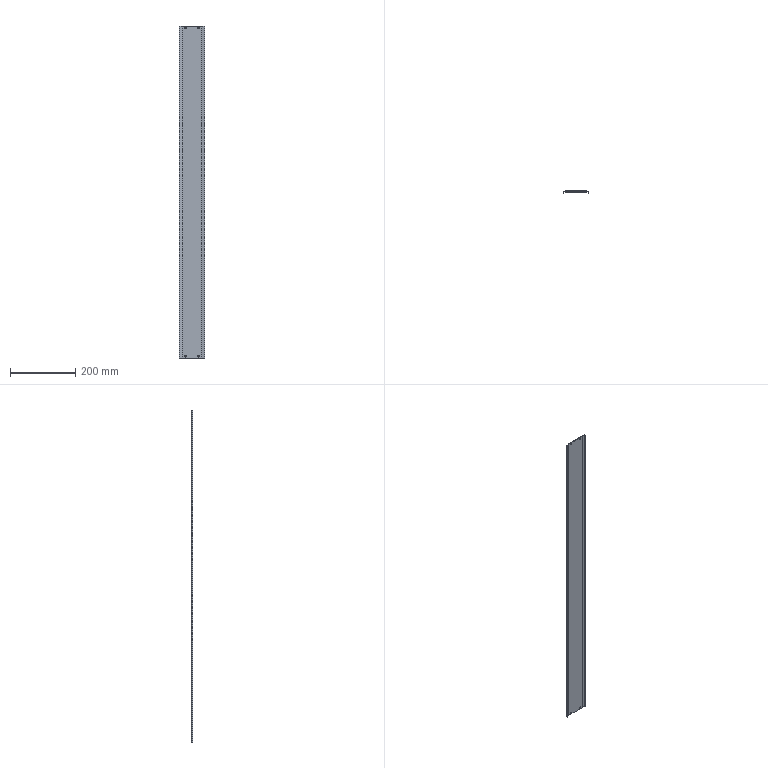Part | SolidWorks | features Cut 1, Extrusion 1, MirrorPattern 1 | 1 solid | 22 faces | box 79 x 6 x 1020 mm | volume 209920 mm3 | plane 14 | cylinder 8 | commonest cylinder face diameters 4.5 x8
STEP:
#1=CARTESIAN_POINT('',(20.,3.5,507.25));
#2=VERTEX_POINT('',#1);
#3=CARTESIAN_POINT('',(20.,3.5,502.75));
#4=VERTEX_POINT('',#3);
#5=CARTESIAN_POINT('',(20.,3.5,505.));
#6=DIRECTION('',(0.,-1.,0.));
#7=DIRECTION('',(0.,0.,1.));
#8=AXIS2_PLACEMENT_3D('',#5,#6,#7);
#9=CIRCLE('',#8,2.25);
#10=EDGE_CURVE('',#2,#4,#9,.T.);
#11=ORIENTED_EDGE('',*,*,#10,.T.);
#12=CARTESIAN_POINT('',(20.,6.,502.75));
#13=VERTEX_POINT('',#12);
#14=CARTESIAN_POINT('',(20.,-14.,502.75));
#15=DIRECTION('',(0.,1.,0.));
#16=VECTOR('',#15,1000.);
#17=LINE('',#14,#16);
#18=EDGE_CURVE('',#4,#13,#17,.T.);
#19=ORIENTED_EDGE('',*,*,#18,.T.);
#20=CARTESIAN_POINT('',(20.,6.,507.25));
#21=VERTEX_POINT('',#20);
#22=CARTESIAN_POINT('',(20.,6.,505.));
#23=DIRECTION('',(0.,-1.,0.));
#24=DIRECTION('',(0.,0.,-1.));
#25=AXIS2_PLACEMENT_3D('',#22,#23,#24);
#26=CIRCLE('',#25,2.25);
#27=EDGE_CURVE('',#21,#13,#26,.T.);
#28=ORIENTED_EDGE('',*,*,#27,.F.);
#29=CARTESIAN_POINT('',(20.,-14.,507.25));
#30=DIRECTION('',(0.,1.,0.));
#31=VECTOR('',#30,1000.);
#32=LINE('',#29,#31);
#33=EDGE_CURVE('',#2,#21,#32,.T.);
#34=ORIENTED_EDGE('',*,*,#33,.F.);
#35=EDGE_LOOP('',(#11,#19,#28,#34));
#36=FACE_OUTER_BOUND('',#35,.T.);
#37=CARTESIAN_POINT('',(20.,-14.,505.));
#38=DIRECTION('',(0.,1.,0.));
#39=DIRECTION('',(0.,0.,1.));
#40=AXIS2_PLACEMENT_3D('',#37,#38,#39);
#41=CYLINDRICAL_SURFACE('',#40,2.25);
#42=ADVANCED_FACE('',(#36),#41,.F.);
#43=CARTESIAN_POINT('',(-20.,3.5,507.25));
#44=VERTEX_POINT('',#43);
#45=CARTESIAN_POINT('',(-20.,3.5,502.75));
#46=VERTEX_POINT('',#45);
#47=CARTESIAN_POINT('',(-20.,3.5,505.));
#48=DIRECTION('',(0.,-1.,0.));
#49=DIRECTION('',(0.,0.,1.));
#50=AXIS2_PLACEMENT_3D('',#47,#48,#49);
#51=CIRCLE('',#50,2.25);
#52=EDGE_CURVE('',#44,#46,#51,.T.);
#53=ORIENTED_EDGE('',*,*,#52,.T.);
#54=CARTESIAN_POINT('',(-20.,6.,502.75));
#55=VERTEX_POINT('',#54);
#56=CARTESIAN_POINT('',(-20.,-14.,502.75));
#57=DIRECTION('',(0.,1.,0.));
#58=VECTOR('',#57,1000.);
#59=LINE('',#56,#58);
#60=EDGE_CURVE('',#46,#55,#59,.T.);
#61=ORIENTED_EDGE('',*,*,#60,.T.);
#62=CARTESIAN_POINT('',(-20.,6.,507.25));
#63=VERTEX_POINT('',#62);
#64=CARTESIAN_POINT('',(-20.,6.,505.));
#65=DIRECTION('',(0.,-1.,0.));
#66=DIRECTION('',(0.,0.,-1.));
#67=AXIS2_PLACEMENT_3D('',#64,#65,#66);
#68=CIRCLE('',#67,2.25);
#69=EDGE_CURVE('',#63,#55,#68,.T.);
#70=ORIENTED_EDGE('',*,*,#69,.F.);
#71=CARTESIAN_POINT('',(-20.,-14.,507.25));
#72=DIRECTION('',(0.,1.,0.));
#73=VECTOR('',#72,1000.);
#74=LINE('',#71,#73);
#75=EDGE_CURVE('',#44,#63,#74,.T.);
#76=ORIENTED_EDGE('',*,*,#75,.F.);
#77=EDGE_LOOP('',(#53,#61,#70,#76));
#78=FACE_OUTER_BOUND('',#77,.T.);
#79=CARTESIAN_POINT('',(-20.,-14.,505.));
#80=DIRECTION('',(0.,1.,0.));
#81=DIRECTION('',(0.,0.,1.));
#82=AXIS2_PLACEMENT_3D('',#79,#80,#81);
#83=CYLINDRICAL_SURFACE('',#82,2.25);
#84=ADVANCED_FACE('',(#78),#83,.F.);
#85=CARTESIAN_POINT('',(20.,3.5,-507.25));
#86=VERTEX_POINT('',#85);
#87=CARTESIAN_POINT('',(20.,3.5,-502.75));
#88=VERTEX_POINT('',#87);
#89=CARTESIAN_POINT('',(20.,3.5,-505.));
#90=DIRECTION('',(0.,1.,0.));
#91=DIRECTION('',(0.,0.,1.));
#92=AXIS2_PLACEMENT_3D('',#89,#90,#91);
#93=CIRCLE('',#92,2.25);
#94=EDGE_CURVE('',#86,#88,#93,.T.);
#95=ORIENTED_EDGE('',*,*,#94,.F.);
#96=CARTESIAN_POINT('',(20.,6.,-507.25));
#97=VERTEX_POINT('',#96);
#98=CARTESIAN_POINT('',(20.,-14.,-507.25));
#99=DIRECTION('',(0.,1.,0.));
#100=VECTOR('',#99,1000.);
#101=LINE('',#98,#100);
#102=EDGE_CURVE('',#86,#97,#101,.T.);
#103=ORIENTED_EDGE('',*,*,#102,.T.);
#104=CARTESIAN_POINT('',(20.,6.,-502.75));
#105=VERTEX_POINT('',#104);
#106=CARTESIAN_POINT('',(20.,6.,-505.));
#107=DIRECTION('',(0.,1.,0.));
#108=DIRECTION('',(0.,0.,1.));
#109=AXIS2_PLACEMENT_3D('',#106,#107,#108);
#110=CIRCLE('',#109,2.25);
#111=EDGE_CURVE('',#97,#105,#110,.T.);
#112=ORIENTED_EDGE('',*,*,#111,.T.);
#113=CARTESIAN_POINT('',(20.,-14.,-502.75));
#114=DIRECTION('',(0.,1.,0.));
#115=VECTOR('',#114,1000.);
#116=LINE('',#113,#115);
#117=EDGE_CURVE('',#88,#105,#116,.T.);
#118=ORIENTED_EDGE('',*,*,#117,.F.);
#119=EDGE_LOOP('',(#95,#103,#112,#118));
#120=FACE_OUTER_BOUND('',#119,.T.);
#121=CARTESIAN_POINT('',(20.,-14.,-505.));
#122=DIRECTION('',(0.,1.,0.));
#123=DIRECTION('',(0.,0.,1.));
#124=AXIS2_PLACEMENT_3D('',#121,#122,#123);
#125=CYLINDRICAL_SURFACE('',#124,2.25);
#126=ADVANCED_FACE('',(#120),#125,.F.);
#127=CARTESIAN_POINT('',(-20.,3.5,-507.25));
#128=VERTEX_POINT('',#127);
#129=CARTESIAN_POINT('',(-20.,3.5,-502.75));
#130=VERTEX_POINT('',#129);
#131=CARTESIAN_POINT('',(-20.,3.5,-505.));
#132=DIRECTION('',(0.,1.,0.));
#133=DIRECTION('',(0.,0.,1.));
#134=AXIS2_PLACEMENT_3D('',#131,#132,#133);
#135=CIRCLE('',#134,2.25);
#136=EDGE_CURVE('',#128,#130,#135,.T.);
#137=ORIENTED_EDGE('',*,*,#136,.F.);
#138=CARTESIAN_POINT('',(-20.,6.,-507.25));
#139=VERTEX_POINT('',#138);
#140=CARTESIAN_POINT('',(-20.,-14.,-507.25));
#141=DIRECTION('',(0.,1.,0.));
#142=VECTOR('',#141,1000.);
#143=LINE('',#140,#142);
#144=EDGE_CURVE('',#128,#139,#143,.T.);
#145=ORIENTED_EDGE('',*,*,#144,.T.);
#146=CARTESIAN_POINT('',(-20.,6.,-502.75));
#147=VERTEX_POINT('',#146);
#148=CARTESIAN_POINT('',(-20.,6.,-505.));
#149=DIRECTION('',(0.,1.,0.));
#150=DIRECTION('',(0.,0.,1.));
#151=AXIS2_PLACEMENT_3D('',#148,#149,#150);
#152=CIRCLE('',#151,2.25);
#153=EDGE_CURVE('',#139,#147,#152,.T.);
#154=ORIENTED_EDGE('',*,*,#153,.T.);
#155=CARTESIAN_POINT('',(-20.,-14.,-502.75));
#156=DIRECTION('',(0.,1.,0.));
#157=VECTOR('',#156,1000.);
#158=LINE('',#155,#157);
#159=EDGE_CURVE('',#130,#147,#158,.T.);
#160=ORIENTED_EDGE('',*,*,#159,.F.);
#161=EDGE_LOOP('',(#137,#145,#154,#160));
#162=FACE_OUTER_BOUND('',#161,.T.);
#163=CARTESIAN_POINT('',(-20.,-14.,-505.));
#164=DIRECTION('',(0.,1.,0.));
#165=DIRECTION('',(0.,0.,1.));
#166=AXIS2_PLACEMENT_3D('',#163,#164,#165);
#167=CYLINDRICAL_SURFACE('',#166,2.25);
#168=ADVANCED_FACE('',(#162),#167,.F.);
#169=CARTESIAN_POINT('',(-37.5,0.,-510.));
#170=VERTEX_POINT('',#169);
#171=CARTESIAN_POINT('',(-37.5,2.122,-510.));
#172=VERTEX_POINT('',#171);
#173=CARTESIAN_POINT('',(-37.5,0.,-510.));
#174=DIRECTION('',(0.,1.,0.));
#175=VECTOR('',#174,1000.);
#176=LINE('',#173,#175);
#177=EDGE_CURVE('',#170,#172,#176,.T.);
#178=ORIENTED_EDGE('',*,*,#177,.T.);
#179=CARTESIAN_POINT('',(-37.5,2.122,510.));
#180=VERTEX_POINT('',#179);
#181=CARTESIAN_POINT('',(-37.5,2.122,510.));
#182=DIRECTION('',(0.,0.,-1.));
#183=VECTOR('',#182,1000.);
#184=LINE('',#181,#183);
#185=EDGE_CURVE('',#180,#172,#184,.T.);
#186=ORIENTED_EDGE('',*,*,#185,.F.);
#187=CARTESIAN_POINT('',(-37.5,0.,510.));
#188=VERTEX_POINT('',#187);
#189=CARTESIAN_POINT('',(-37.5,0.,510.));
#190=DIRECTION('',(0.,1.,0.));
#191=VECTOR('',#190,1000.);
#192=LINE('',#189,#191);
#193=EDGE_CURVE('',#188,#180,#192,.T.);
#194=ORIENTED_EDGE('',*,*,#193,.F.);
#195=CARTESIAN_POINT('',(-37.5,0.,510.));
#196=DIRECTION('',(0.,0.,-1.));
#197=VECTOR('',#196,1000.);
#198=LINE('',#195,#197);
#199=EDGE_CURVE('',#188,#170,#198,.T.);
#200=ORIENTED_EDGE('',*,*,#199,.T.);
#201=EDGE_LOOP('',(#178,#186,#194,#200));
#202=FACE_OUTER_BOUND('',#201,.T.);
#203=CARTESIAN_POINT('',(-37.5,0.,510.));
#204=DIRECTION('',(-1.,0.,0.));
#205=DIRECTION('',(0.,0.,1.));
#206=AXIS2_PLACEMENT_3D('',#203,#204,#205);
#207=PLANE('',#206);
#208=ADVANCED_FACE('',(#202),#207,.F.);
#209=CARTESIAN_POINT('',(-29.8,3.5,-510.));
#210=VERTEX_POINT('',#209);
#211=CARTESIAN_POINT('',(-37.5,2.122,-510.));
#212=DIRECTION('',(0.9844,0.1761,0.));
#213=VECTOR('',#212,1000.);
#214=LINE('',#211,#213);
#215=EDGE_CURVE('',#172,#210,#214,.T.);
#216=ORIENTED_EDGE('',*,*,#215,.T.);
#217=CARTESIAN_POINT('',(-29.8,3.5,510.));
#218=VERTEX_POINT('',#217);
#219=CARTESIAN_POINT('',(-29.8,3.5,510.));
#220=DIRECTION('',(0.,0.,-1.));
#221=VECTOR('',#220,1000.);
#222=LINE('',#219,#221);
#223=EDGE_CURVE('',#218,#210,#222,.T.);
#224=ORIENTED_EDGE('',*,*,#223,.F.);
#225=CARTESIAN_POINT('',(-37.5,2.122,510.));
#226=DIRECTION('',(0.9844,0.1761,0.));
#227=VECTOR('',#226,1000.);
#228=LINE('',#225,#227);
#229=EDGE_CURVE('',#180,#218,#228,.T.);
#230=ORIENTED_EDGE('',*,*,#229,.F.);
#231=ORIENTED_EDGE('',*,*,#185,.T.);
#232=EDGE_LOOP('',(#216,#224,#230,#231));
#233=FACE_OUTER_BOUND('',#232,.T.);
#234=CARTESIAN_POINT('',(-37.5,2.122,510.));
#235=DIRECTION('',(-0.1761,0.9844,0.));
#236=DIRECTION('',(-0.9844,-0.1761,0.));
#237=AXIS2_PLACEMENT_3D('',#234,#235,#236);
#238=PLANE('',#237);
#239=ADVANCED_FACE('',(#233),#238,.F.);
#240=ORIENTED_EDGE('',*,*,#10,.F.);
#241=CARTESIAN_POINT('',(20.,3.5,505.));
#242=DIRECTION('',(0.,-1.,0.));
#243=DIRECTION('',(0.,0.,1.));
#244=AXIS2_PLACEMENT_3D('',#241,#242,#243);
#245=CIRCLE('',#244,2.25);
#246=EDGE_CURVE('',#4,#2,#245,.T.);
#247=ORIENTED_EDGE('',*,*,#246,.F.);
#248=EDGE_LOOP('',(#240,#247));
#249=FACE_BOUND('',#248,.T.);
#250=ORIENTED_EDGE('',*,*,#52,.F.);
#251=CARTESIAN_POINT('',(-20.,3.5,505.));
#252=DIRECTION('',(0.,-1.,0.));
#253=DIRECTION('',(0.,0.,1.));
#254=AXIS2_PLACEMENT_3D('',#251,#252,#253);
#255=CIRCLE('',#254,2.25);
#256=EDGE_CURVE('',#46,#44,#255,.T.);
#257=ORIENTED_EDGE('',*,*,#256,.F.);
#258=EDGE_LOOP('',(#250,#257));
#259=FACE_BOUND('',#258,.T.);
#260=CARTESIAN_POINT('',(20.,3.5,-505.));
#261=DIRECTION('',(0.,1.,0.));
#262=DIRECTION('',(0.,0.,1.));
#263=AXIS2_PLACEMENT_3D('',#260,#261,#262);
#264=CIRCLE('',#263,2.25);
#265=EDGE_CURVE('',#88,#86,#264,.T.);
#266=ORIENTED_EDGE('',*,*,#265,.T.);
#267=ORIENTED_EDGE('',*,*,#94,.T.);
#268=EDGE_LOOP('',(#266,#267));
#269=FACE_BOUND('',#268,.T.);
#270=CARTESIAN_POINT('',(-20.,3.5,-505.));
#271=DIRECTION('',(0.,1.,0.));
#272=DIRECTION('',(0.,0.,1.));
#273=AXIS2_PLACEMENT_3D('',#270,#271,#272);
#274=CIRCLE('',#273,2.25);
#275=EDGE_CURVE('',#130,#128,#274,.T.);
#276=ORIENTED_EDGE('',*,*,#275,.T.);
#277=ORIENTED_EDGE('',*,*,#136,.T.);
#278=EDGE_LOOP('',(#276,#277));
#279=FACE_BOUND('',#278,.T.);
#280=CARTESIAN_POINT('',(29.8,3.5,-510.));
#281=VERTEX_POINT('',#280);
#282=CARTESIAN_POINT('',(-29.8,3.5,-510.));
#283=DIRECTION('',(1.,0.,0.));
#284=VECTOR('',#283,1000.);
#285=LINE('',#282,#284);
#286=EDGE_CURVE('',#210,#281,#285,.T.);
#287=ORIENTED_EDGE('',*,*,#286,.T.);
#288=CARTESIAN_POINT('',(29.8,3.5,510.));
#289=VERTEX_POINT('',#288);
#290=CARTESIAN_POINT('',(29.8,3.5,510.));
#291=DIRECTION('',(0.,0.,-1.));
#292=VECTOR('',#291,1000.);
#293=LINE('',#290,#292);
#294=EDGE_CURVE('',#289,#281,#293,.T.);
#295=ORIENTED_EDGE('',*,*,#294,.F.);
#296=CARTESIAN_POINT('',(-29.8,3.5,510.));
#297=DIRECTION('',(1.,0.,0.));
#298=VECTOR('',#297,1000.);
#299=LINE('',#296,#298);
#300=EDGE_CURVE('',#218,#289,#299,.T.);
#301=ORIENTED_EDGE('',*,*,#300,.F.);
#302=ORIENTED_EDGE('',*,*,#223,.T.);
#303=EDGE_LOOP('',(#287,#295,#301,#302));
#304=FACE_OUTER_BOUND('',#303,.T.);
#305=CARTESIAN_POINT('',(-29.8,3.5,510.));
#306=DIRECTION('',(0.,1.,0.));
#307=DIRECTION('',(0.,0.,1.));
#308=AXIS2_PLACEMENT_3D('',#305,#306,#307);
#309=PLANE('',#308);
#310=ADVANCED_FACE('',(#249,#259,#269,#279,#304),#309,.F.);
#311=CARTESIAN_POINT('',(37.5,2.122,-510.));
#312=VERTEX_POINT('',#311);
#313=CARTESIAN_POINT('',(37.5,2.122,-510.));
#314=DIRECTION('',(0.9844,-0.1761,0.));
#315=VECTOR('',#314,1000.);
#316=LINE('',#313,#315);
#317=EDGE_CURVE('',#281,#312,#316,.T.);
#318=ORIENTED_EDGE('',*,*,#317,.T.);
#319=CARTESIAN_POINT('',(37.5,2.122,510.));
#320=VERTEX_POINT('',#319);
#321=CARTESIAN_POINT('',(37.5,2.122,510.));
#322=DIRECTION('',(0.,0.,-1.));
#323=VECTOR('',#322,1000.);
#324=LINE('',#321,#323);
#325=EDGE_CURVE('',#320,#312,#324,.T.);
#326=ORIENTED_EDGE('',*,*,#325,.F.);
#327=CARTESIAN_POINT('',(37.5,2.122,510.));
#328=DIRECTION('',(0.9844,-0.1761,0.));
#329=VECTOR('',#328,1000.);
#330=LINE('',#327,#329);
#331=EDGE_CURVE('',#289,#320,#330,.T.);
#332=ORIENTED_EDGE('',*,*,#331,.F.);
#333=ORIENTED_EDGE('',*,*,#294,.T.);
#334=EDGE_LOOP('',(#318,#326,#332,#333));
#335=FACE_OUTER_BOUND('',#334,.T.);
#336=CARTESIAN_POINT('',(37.5,2.122,510.));
#337=DIRECTION('',(0.1761,0.9844,0.));
#338=DIRECTION('',(-0.9844,0.1761,0.));
#339=AXIS2_PLACEMENT_3D('',#336,#337,#338);
#340=PLANE('',#339);
#341=ADVANCED_FACE('',(#335),#340,.F.);
#342=CARTESIAN_POINT('',(37.5,0.,-510.));
#343=VERTEX_POINT('',#342);
#344=CARTESIAN_POINT('',(37.5,0.,-510.));
#345=DIRECTION('',(0.,-1.,0.));
#346=VECTOR('',#345,1000.);
#347=LINE('',#344,#346);
#348=EDGE_CURVE('',#312,#343,#347,.T.);
#349=ORIENTED_EDGE('',*,*,#348,.T.);
#350=CARTESIAN_POINT('',(37.5,0.,510.));
#351=VERTEX_POINT('',#350);
#352=CARTESIAN_POINT('',(37.5,0.,510.));
#353=DIRECTION('',(0.,0.,-1.));
#354=VECTOR('',#353,1000.);
#355=LINE('',#352,#354);
#356=EDGE_CURVE('',#351,#343,#355,.T.);
#357=ORIENTED_EDGE('',*,*,#356,.F.);
#358=CARTESIAN_POINT('',(37.5,0.,510.));
#359=DIRECTION('',(0.,-1.,0.));
#360=VECTOR('',#359,1000.);
#361=LINE('',#358,#360);
#362=EDGE_CURVE('',#320,#351,#361,.T.);
#363=ORIENTED_EDGE('',*,*,#362,.F.);
#364=ORIENTED_EDGE('',*,*,#325,.T.);
#365=EDGE_LOOP('',(#349,#357,#363,#364));
#366=FACE_OUTER_BOUND('',#365,.T.);
#367=CARTESIAN_POINT('',(37.5,0.,510.));
#368=DIRECTION('',(1.,0.,0.));
#369=DIRECTION('',(0.,0.,-1.));
#370=AXIS2_PLACEMENT_3D('',#367,#368,#369);
#371=PLANE('',#370);
#372=ADVANCED_FACE('',(#366),#371,.F.);
#373=CARTESIAN_POINT('',(39.5,0.,-510.));
#374=VERTEX_POINT('',#373);
#375=CARTESIAN_POINT('',(37.5,0.,-510.));
#376=DIRECTION('',(1.,0.,0.));
#377=VECTOR('',#376,1000.);
#378=LINE('',#375,#377);
#379=EDGE_CURVE('',#343,#374,#378,.T.);
#380=ORIENTED_EDGE('',*,*,#379,.T.);
#381=CARTESIAN_POINT('',(39.5,0.,510.));
#382=VERTEX_POINT('',#381);
#383=CARTESIAN_POINT('',(39.5,0.,510.));
#384=DIRECTION('',(0.,0.,-1.));
#385=VECTOR('',#384,1000.);
#386=LINE('',#383,#385);
#387=EDGE_CURVE('',#382,#374,#386,.T.);
#388=ORIENTED_EDGE('',*,*,#387,.F.);
#389=CARTESIAN_POINT('',(37.5,0.,510.));
#390=DIRECTION('',(1.,0.,0.));
#391=VECTOR('',#390,1000.);
#392=LINE('',#389,#391);
#393=EDGE_CURVE('',#351,#382,#392,.T.);
#394=ORIENTED_EDGE('',*,*,#393,.F.);
#395=ORIENTED_EDGE('',*,*,#356,.T.);
#396=EDGE_LOOP('',(#380,#388,#394,#395));
#397=FACE_OUTER_BOUND('',#396,.T.);
#398=CARTESIAN_POINT('',(37.5,0.,510.));
#399=DIRECTION('',(0.,1.,0.));
#400=DIRECTION('',(-1.,0.,0.));
#401=AXIS2_PLACEMENT_3D('',#398,#399,#400);
#402=PLANE('',#401);
#403=ADVANCED_FACE('',(#397),#402,.F.);
#404=CARTESIAN_POINT('',(39.5,4.3,-510.));
#405=VERTEX_POINT('',#404);
#406=CARTESIAN_POINT('',(39.5,0.,-510.));
#407=DIRECTION('',(0.,1.,0.));
#408=VECTOR('',#407,1000.);
#409=LINE('',#406,#408);
#410=EDGE_CURVE('',#374,#405,#409,.T.);
#411=ORIENTED_EDGE('',*,*,#410,.T.);
#412=CARTESIAN_POINT('',(39.5,4.3,510.));
#413=VERTEX_POINT('',#412);
#414=CARTESIAN_POINT('',(39.5,4.3,510.));
#415=DIRECTION('',(0.,0.,-1.));
#416=VECTOR('',#415,1000.);
#417=LINE('',#414,#416);
#418=EDGE_CURVE('',#413,#405,#417,.T.);
#419=ORIENTED_EDGE('',*,*,#418,.F.);
#420=CARTESIAN_POINT('',(39.5,0.,510.));
#421=DIRECTION('',(0.,1.,0.));
#422=VECTOR('',#421,1000.);
#423=LINE('',#420,#422);
#424=EDGE_CURVE('',#382,#413,#423,.T.);
#425=ORIENTED_EDGE('',*,*,#424,.F.);
#426=ORIENTED_EDGE('',*,*,#387,.T.);
#427=EDGE_LOOP('',(#411,#419,#425,#426));
#428=FACE_OUTER_BOUND('',#427,.T.);
#429=CARTESIAN_POINT('',(39.5,0.,510.));
#430=DIRECTION('',(-1.,0.,0.));
#431=DIRECTION('',(0.,0.,1.));
#432=AXIS2_PLACEMENT_3D('',#429,#430,#431);
#433=PLANE('',#432);
#434=ADVANCED_FACE('',(#428),#433,.F.);
#435=CARTESIAN_POINT('',(30.,6.,-510.));
#436=VERTEX_POINT('',#435);
#437=CARTESIAN_POINT('',(39.5,4.3,-510.));
#438=DIRECTION('',(-0.9844,0.1761,0.));
#439=VECTOR('',#438,1000.);
#440=LINE('',#437,#439);
#441=EDGE_CURVE('',#405,#436,#440,.T.);
#442=ORIENTED_EDGE('',*,*,#441,.T.);
#443=CARTESIAN_POINT('',(30.,6.,510.));
#444=VERTEX_POINT('',#443);
#445=CARTESIAN_POINT('',(30.,6.,510.));
#446=DIRECTION('',(0.,0.,-1.));
#447=VECTOR('',#446,1000.);
#448=LINE('',#445,#447);
#449=EDGE_CURVE('',#444,#436,#448,.T.);
#450=ORIENTED_EDGE('',*,*,#449,.F.);
#451=CARTESIAN_POINT('',(39.5,4.3,510.));
#452=DIRECTION('',(-0.9844,0.1761,0.));
#453=VECTOR('',#452,1000.);
#454=LINE('',#451,#453);
#455=EDGE_CURVE('',#413,#444,#454,.T.);
#456=ORIENTED_EDGE('',*,*,#455,.F.);
#457=ORIENTED_EDGE('',*,*,#418,.T.);
#458=EDGE_LOOP('',(#442,#450,#456,#457));
#459=FACE_OUTER_BOUND('',#458,.T.);
#460=CARTESIAN_POINT('',(39.5,4.3,510.));
#461=DIRECTION('',(-0.1761,-0.9844,0.));
#462=DIRECTION('',(0.9844,-0.1761,0.));
#463=AXIS2_PLACEMENT_3D('',#460,#461,#462);
#464=PLANE('',#463);
#465=ADVANCED_FACE('',(#459),#464,.F.);
#466=ORIENTED_EDGE('',*,*,#27,.T.);
#467=CARTESIAN_POINT('',(20.,6.,505.));
#468=DIRECTION('',(0.,-1.,0.));
#469=DIRECTION('',(0.,0.,-1.));
#470=AXIS2_PLACEMENT_3D('',#467,#468,#469);
#471=CIRCLE('',#470,2.25);
#472=EDGE_CURVE('',#13,#21,#471,.T.);
#473=ORIENTED_EDGE('',*,*,#472,.T.);
#474=EDGE_LOOP('',(#466,#473));
#475=FACE_BOUND('',#474,.T.);
#476=ORIENTED_EDGE('',*,*,#69,.T.);
#477=CARTESIAN_POINT('',(-20.,6.,505.));
#478=DIRECTION('',(0.,-1.,0.));
#479=DIRECTION('',(0.,0.,-1.));
#480=AXIS2_PLACEMENT_3D('',#477,#478,#479);
#481=CIRCLE('',#480,2.25);
#482=EDGE_CURVE('',#55,#63,#481,.T.);
#483=ORIENTED_EDGE('',*,*,#482,.T.);
#484=EDGE_LOOP('',(#476,#483));
#485=FACE_BOUND('',#484,.T.);
#486=CARTESIAN_POINT('',(20.,6.,-505.));
#487=DIRECTION('',(0.,1.,0.));
#488=DIRECTION('',(0.,0.,1.));
#489=AXIS2_PLACEMENT_3D('',#486,#487,#488);
#490=CIRCLE('',#489,2.25);
#491=EDGE_CURVE('',#105,#97,#490,.T.);
#492=ORIENTED_EDGE('',*,*,#491,.F.);
#493=ORIENTED_EDGE('',*,*,#111,.F.);
#494=EDGE_LOOP('',(#492,#493));
#495=FACE_BOUND('',#494,.T.);
#496=CARTESIAN_POINT('',(-20.,6.,-505.));
#497=DIRECTION('',(0.,1.,0.));
#498=DIRECTION('',(0.,0.,1.));
#499=AXIS2_PLACEMENT_3D('',#496,#497,#498);
#500=CIRCLE('',#499,2.25);
#501=EDGE_CURVE('',#147,#139,#500,.T.);
#502=ORIENTED_EDGE('',*,*,#501,.F.);
#503=ORIENTED_EDGE('',*,*,#153,.F.);
#504=EDGE_LOOP('',(#502,#503));
#505=FACE_BOUND('',#504,.T.);
#506=CARTESIAN_POINT('',(-30.,6.,-510.));
#507=VERTEX_POINT('',#506);
#508=CARTESIAN_POINT('',(-30.,6.,-510.));
#509=DIRECTION('',(-1.,0.,0.));
#510=VECTOR('',#509,1000.);
#511=LINE('',#508,#510);
#512=EDGE_CURVE('',#436,#507,#511,.T.);
#513=ORIENTED_EDGE('',*,*,#512,.T.);
#514=CARTESIAN_POINT('',(-30.,6.,510.));
#515=VERTEX_POINT('',#514);
#516=CARTESIAN_POINT('',(-30.,6.,510.));
#517=DIRECTION('',(0.,0.,-1.));
#518=VECTOR('',#517,1000.);
#519=LINE('',#516,#518);
#520=EDGE_CURVE('',#515,#507,#519,.T.);
#521=ORIENTED_EDGE('',*,*,#520,.F.);
#522=CARTESIAN_POINT('',(-30.,6.,510.));
#523=DIRECTION('',(-1.,0.,0.));
#524=VECTOR('',#523,1000.);
#525=LINE('',#522,#524);
#526=EDGE_CURVE('',#444,#515,#525,.T.);
#527=ORIENTED_EDGE('',*,*,#526,.F.);
#528=ORIENTED_EDGE('',*,*,#449,.T.);
#529=EDGE_LOOP('',(#513,#521,#527,#528));
#530=FACE_OUTER_BOUND('',#529,.T.);
#531=CARTESIAN_POINT('',(-30.,6.,510.));
#532=DIRECTION('',(0.,-1.,0.));
#533=DIRECTION('',(0.,0.,-1.));
#534=AXIS2_PLACEMENT_3D('',#531,#532,#533);
#535=PLANE('',#534);
#536=ADVANCED_FACE('',(#475,#485,#495,#505,#530),#535,.F.);
#537=CARTESIAN_POINT('',(-39.5,4.3,-510.));
#538=VERTEX_POINT('',#537);
#539=CARTESIAN_POINT('',(-39.5,4.3,-510.));
#540=DIRECTION('',(-0.9844,-0.1761,0.));
#541=VECTOR('',#540,1000.);
#542=LINE('',#539,#541);
#543=EDGE_CURVE('',#507,#538,#542,.T.);
#544=ORIENTED_EDGE('',*,*,#543,.T.);
#545=CARTESIAN_POINT('',(-39.5,4.3,510.));
#546=VERTEX_POINT('',#545);
#547=CARTESIAN_POINT('',(-39.5,4.3,510.));
#548=DIRECTION('',(0.,0.,-1.));
#549=VECTOR('',#548,1000.);
#550=LINE('',#547,#549);
#551=EDGE_CURVE('',#546,#538,#550,.T.);
#552=ORIENTED_EDGE('',*,*,#551,.F.);
#553=CARTESIAN_POINT('',(-39.5,4.3,510.));
#554=DIRECTION('',(-0.9844,-0.1761,0.));
#555=VECTOR('',#554,1000.);
#556=LINE('',#553,#555);
#557=EDGE_CURVE('',#515,#546,#556,.T.);
#558=ORIENTED_EDGE('',*,*,#557,.F.);
#559=ORIENTED_EDGE('',*,*,#520,.T.);
#560=EDGE_LOOP('',(#544,#552,#558,#559));
#561=FACE_OUTER_BOUND('',#560,.T.);
#562=CARTESIAN_POINT('',(-39.5,4.3,510.));
#563=DIRECTION('',(0.1761,-0.9844,0.));
#564=DIRECTION('',(0.9844,0.1761,0.));
#565=AXIS2_PLACEMENT_3D('',#562,#563,#564);
#566=PLANE('',#565);
#567=ADVANCED_FACE('',(#561),#566,.F.);
#568=CARTESIAN_POINT('',(-39.5,0.,-510.));
#569=VERTEX_POINT('',#568);
#570=CARTESIAN_POINT('',(-39.5,0.,-510.));
#571=DIRECTION('',(0.,-1.,0.));
#572=VECTOR('',#571,1000.);
#573=LINE('',#570,#572);
#574=EDGE_CURVE('',#538,#569,#573,.T.);
#575=ORIENTED_EDGE('',*,*,#574,.T.);
#576=CARTESIAN_POINT('',(-39.5,0.,510.));
#577=VERTEX_POINT('',#576);
#578=CARTESIAN_POINT('',(-39.5,0.,510.));
#579=DIRECTION('',(0.,0.,-1.));
#580=VECTOR('',#579,1000.);
#581=LINE('',#578,#580);
#582=EDGE_CURVE('',#577,#569,#581,.T.);
#583=ORIENTED_EDGE('',*,*,#582,.F.);
#584=CARTESIAN_POINT('',(-39.5,0.,510.));
#585=DIRECTION('',(0.,-1.,0.));
#586=VECTOR('',#585,1000.);
#587=LINE('',#584,#586);
#588=EDGE_CURVE('',#546,#577,#587,.T.);
#589=ORIENTED_EDGE('',*,*,#588,.F.);
#590=ORIENTED_EDGE('',*,*,#551,.T.);
#591=EDGE_LOOP('',(#575,#583,#589,#590));
#592=FACE_OUTER_BOUND('',#591,.T.);
#593=CARTESIAN_POINT('',(-39.5,0.,510.));
#594=DIRECTION('',(1.,0.,0.));
#595=DIRECTION('',(0.,0.,-1.));
#596=AXIS2_PLACEMENT_3D('',#593,#594,#595);
#597=PLANE('',#596);
#598=ADVANCED_FACE('',(#592),#597,.F.);
#599=CARTESIAN_POINT('',(-37.5,0.,-510.));
#600=DIRECTION('',(1.,0.,0.));
#601=VECTOR('',#600,1000.);
#602=LINE('',#599,#601);
#603=EDGE_CURVE('',#569,#170,#602,.T.);
#604=ORIENTED_EDGE('',*,*,#603,.T.);
#605=ORIENTED_EDGE('',*,*,#199,.F.);
#606=CARTESIAN_POINT('',(-37.5,0.,510.));
#607=DIRECTION('',(1.,0.,0.));
#608=VECTOR('',#607,1000.);
#609=LINE('',#606,#608);
#610=EDGE_CURVE('',#577,#188,#609,.T.);
#611=ORIENTED_EDGE('',*,*,#610,.F.);
#612=ORIENTED_EDGE('',*,*,#582,.T.);
#613=EDGE_LOOP('',(#604,#605,#611,#612));
#614=FACE_OUTER_BOUND('',#613,.T.);
#615=CARTESIAN_POINT('',(-37.5,0.,510.));
#616=DIRECTION('',(0.,1.,0.));
#617=DIRECTION('',(-1.,0.,0.));
#618=AXIS2_PLACEMENT_3D('',#615,#616,#617);
#619=PLANE('',#618);
#620=ADVANCED_FACE('',(#614),#619,.F.);
#621=ORIENTED_EDGE('',*,*,#193,.T.);
#622=ORIENTED_EDGE('',*,*,#229,.T.);
#623=ORIENTED_EDGE('',*,*,#300,.T.);
#624=ORIENTED_EDGE('',*,*,#331,.T.);
#625=ORIENTED_EDGE('',*,*,#362,.T.);
#626=ORIENTED_EDGE('',*,*,#393,.T.);
#627=ORIENTED_EDGE('',*,*,#424,.T.);
#628=ORIENTED_EDGE('',*,*,#455,.T.);
#629=ORIENTED_EDGE('',*,*,#526,.T.);
#630=ORIENTED_EDGE('',*,*,#557,.T.);
#631=ORIENTED_EDGE('',*,*,#588,.T.);
#632=ORIENTED_EDGE('',*,*,#610,.T.);
#633=EDGE_LOOP('',(#621,#622,#623,#624,#625,#626,#627,#628,#629,#630,#631,#632));
#634=FACE_OUTER_BOUND('',#633,.T.);
#635=CARTESIAN_POINT('',(0.,0.,510.));
#636=DIRECTION('',(0.,0.,-1.));
#637=DIRECTION('',(-1.,0.,0.));
#638=AXIS2_PLACEMENT_3D('',#635,#636,#637);
#639=PLANE('',#638);
#640=ADVANCED_FACE('',(#634),#639,.F.);
#641=ORIENTED_EDGE('',*,*,#177,.F.);
#642=ORIENTED_EDGE('',*,*,#603,.F.);
#643=ORIENTED_EDGE('',*,*,#574,.F.);
#644=ORIENTED_EDGE('',*,*,#543,.F.);
#645=ORIENTED_EDGE('',*,*,#512,.F.);
#646=ORIENTED_EDGE('',*,*,#441,.F.);
#647=ORIENTED_EDGE('',*,*,#410,.F.);
#648=ORIENTED_EDGE('',*,*,#379,.F.);
#649=ORIENTED_EDGE('',*,*,#348,.F.);
#650=ORIENTED_EDGE('',*,*,#317,.F.);
#651=ORIENTED_EDGE('',*,*,#286,.F.);
#652=ORIENTED_EDGE('',*,*,#215,.F.);
#653=EDGE_LOOP('',(#641,#642,#643,#644,#645,#646,#647,#648,#649,#650,#651,#652));
#654=FACE_OUTER_BOUND('',#653,.T.);
#655=CARTESIAN_POINT('',(0.,0.,-510.));
#656=DIRECTION('',(0.,0.,-1.));
#657=DIRECTION('',(-1.,0.,0.));
#658=AXIS2_PLACEMENT_3D('',#655,#656,#657);
#659=PLANE('',#658);
#660=ADVANCED_FACE('',(#654),#659,.T.);
#661=ORIENTED_EDGE('',*,*,#144,.F.);
#662=ORIENTED_EDGE('',*,*,#275,.F.);
#663=ORIENTED_EDGE('',*,*,#159,.T.);
#664=ORIENTED_EDGE('',*,*,#501,.T.);
#665=EDGE_LOOP('',(#661,#662,#663,#664));
#666=FACE_OUTER_BOUND('',#665,.T.);
#667=CARTESIAN_POINT('',(-20.,-14.,-505.));
#668=DIRECTION('',(0.,1.,0.));
#669=DIRECTION('',(0.,0.,1.));
#670=AXIS2_PLACEMENT_3D('',#667,#668,#669);
#671=CYLINDRICAL_SURFACE('',#670,2.25);
#672=ADVANCED_FACE('',(#666),#671,.F.);
#673=ORIENTED_EDGE('',*,*,#102,.F.);
#674=ORIENTED_EDGE('',*,*,#265,.F.);
#675=ORIENTED_EDGE('',*,*,#117,.T.);
#676=ORIENTED_EDGE('',*,*,#491,.T.);
#677=EDGE_LOOP('',(#673,#674,#675,#676));
#678=FACE_OUTER_BOUND('',#677,.T.);
#679=CARTESIAN_POINT('',(20.,-14.,-505.));
#680=DIRECTION('',(0.,1.,0.));
#681=DIRECTION('',(0.,0.,1.));
#682=AXIS2_PLACEMENT_3D('',#679,#680,#681);
#683=CYLINDRICAL_SURFACE('',#682,2.25);
#684=ADVANCED_FACE('',(#678),#683,.F.);
#685=ORIENTED_EDGE('',*,*,#60,.F.);
#686=ORIENTED_EDGE('',*,*,#256,.T.);
#687=ORIENTED_EDGE('',*,*,#75,.T.);
#688=ORIENTED_EDGE('',*,*,#482,.F.);
#689=EDGE_LOOP('',(#685,#686,#687,#688));
#690=FACE_OUTER_BOUND('',#689,.T.);
#691=CARTESIAN_POINT('',(-20.,-14.,505.));
#692=DIRECTION('',(0.,1.,0.));
#693=DIRECTION('',(0.,0.,1.));
#694=AXIS2_PLACEMENT_3D('',#691,#692,#693);
#695=CYLINDRICAL_SURFACE('',#694,2.25);
#696=ADVANCED_FACE('',(#690),#695,.F.);
#697=ORIENTED_EDGE('',*,*,#18,.F.);
#698=ORIENTED_EDGE('',*,*,#246,.T.);
#699=ORIENTED_EDGE('',*,*,#33,.T.);
#700=ORIENTED_EDGE('',*,*,#472,.F.);
#701=EDGE_LOOP('',(#697,#698,#699,#700));
#702=FACE_OUTER_BOUND('',#701,.T.);
#703=CARTESIAN_POINT('',(20.,-14.,505.));
#704=DIRECTION('',(0.,1.,0.));
#705=DIRECTION('',(0.,0.,1.));
#706=AXIS2_PLACEMENT_3D('',#703,#704,#705);
#707=CYLINDRICAL_SURFACE('',#706,2.25);
#708=ADVANCED_FACE('',(#702),#707,.F.);
#709=CLOSED_SHELL('',(#42,#84,#126,#168,#208,#239,#310,#341,#372,#403,#434,#465,#536,#567,#598,#620,#640,#660,#672,#684,#696,#708));
#710=MANIFOLD_SOLID_BREP('',#709);
#711=CARTESIAN_POINT('',(0.,0.,0.));
#712=DIRECTION('',(0.,0.,1.));
#713=DIRECTION('',(1.,0.,0.));
#714=AXIS2_PLACEMENT_3D('',#711,#712,#713);
#715=(LENGTH_UNIT()NAMED_UNIT(*)SI_UNIT(.MILLI.,.METRE.));
#716=UNCERTAINTY_MEASURE_WITH_UNIT(LENGTH_MEASURE(0.00001),#715,'','');
#717=(NAMED_UNIT(*)PLANE_ANGLE_UNIT()SI_UNIT($,.RADIAN.));
#718=(NAMED_UNIT(*)SI_UNIT($,.STERADIAN.)SOLID_ANGLE_UNIT());
#719=(GEOMETRIC_REPRESENTATION_CONTEXT(3)GLOBAL_UNCERTAINTY_ASSIGNED_CONTEXT((#716))GLOBAL_UNIT_ASSIGNED_CONTEXT((#715,#717,#718))REPRESENTATION_CONTEXT('',''));
#720=ADVANCED_BREP_SHAPE_REPRESENTATION('',(#710,#714),#719);